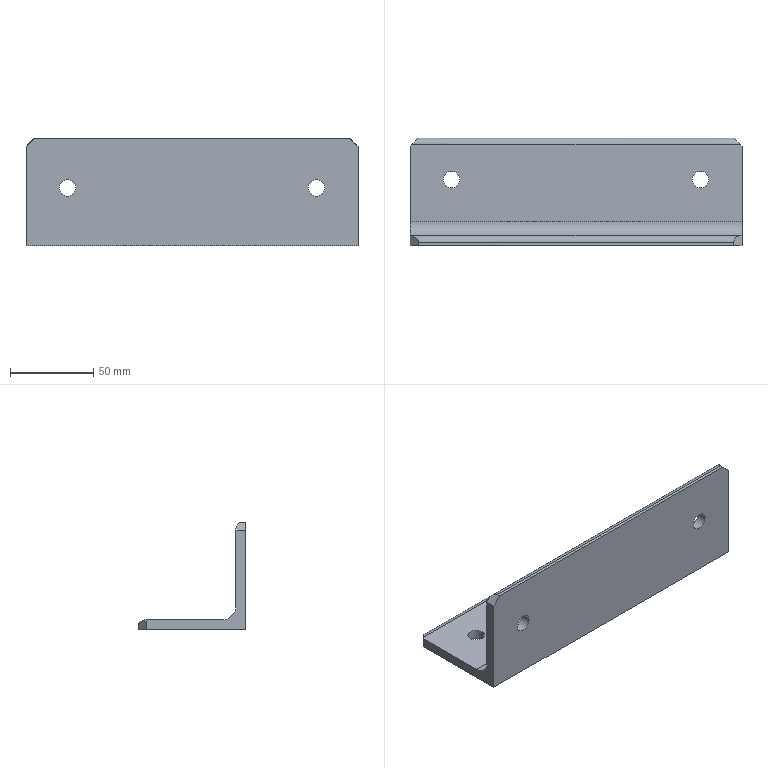Part | STEP file | J452-EBZ05-22-08 | 1 solid | 23 faces | box 200 x 65 x 65 mm | volume 148399 mm3 | plane 12 | cylinder 11 | commonest cylinder face diameters 10 x8 8 x2 17 x1